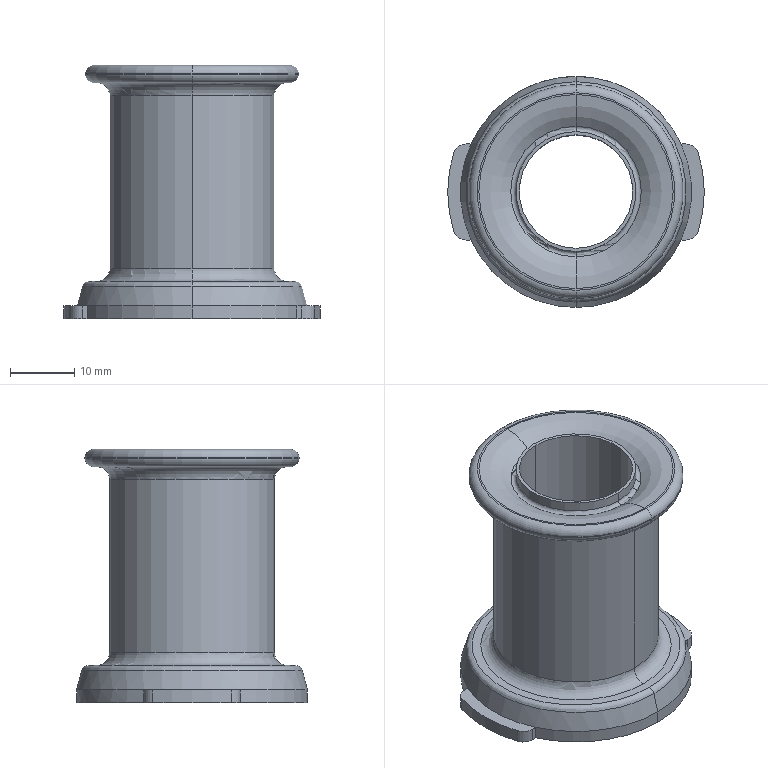Part | SolidWorks | features BaseBody 1 | 1 solid | 51 faces | box 40 x 36 x 39.5 mm | volume 12667 mm3 | cylinder 19 | torus 18 | plane 12 | cone 2 | commonest cylinder face diameters 4 x4 36 x3 17.7 x2 18.7 x2 25.7 x2 33.4 x2
STEP:
#1=CARTESIAN_POINT('',(2003.,227.,823.));
#2=VERTEX_POINT('',#1);
#3=CARTESIAN_POINT('',(2019.363,237.5,823.));
#4=VERTEX_POINT('',#3);
#5=CARTESIAN_POINT('',(2003.,245.,823.));
#6=DIRECTION('',(0.,0.,1.));
#7=DIRECTION('',(0.,-1.,0.));
#8=AXIS2_PLACEMENT_3D('',#5,#6,#7);
#9=CIRCLE('',#8,18.);
#10=EDGE_CURVE('',#2,#4,#9,.T.);
#11=ORIENTED_EDGE('',*,*,#10,.F.);
#12=CARTESIAN_POINT('',(2003.,227.,821.));
#13=VERTEX_POINT('',#12);
#14=CARTESIAN_POINT('',(2003.,227.,862.625));
#15=DIRECTION('',(0.,0.,-1.));
#16=VECTOR('',#15,1000.);
#17=LINE('',#14,#16);
#18=EDGE_CURVE('',#2,#13,#17,.T.);
#19=ORIENTED_EDGE('',*,*,#18,.T.);
#20=CARTESIAN_POINT('',(2019.363,237.5,821.));
#21=VERTEX_POINT('',#20);
#22=CARTESIAN_POINT('',(2003.,245.,821.));
#23=DIRECTION('',(0.,0.,-1.));
#24=DIRECTION('',(0.9091,-0.4167,0.));
#25=AXIS2_PLACEMENT_3D('',#22,#23,#24);
#26=CIRCLE('',#25,18.);
#27=EDGE_CURVE('',#21,#13,#26,.T.);
#28=ORIENTED_EDGE('',*,*,#27,.F.);
#29=CARTESIAN_POINT('',(2019.363,237.5,823.));
#30=DIRECTION('',(0.,0.,-1.));
#31=VECTOR('',#30,1000.);
#32=LINE('',#29,#31);
#33=EDGE_CURVE('',#4,#21,#32,.T.);
#34=ORIENTED_EDGE('',*,*,#33,.F.);
#35=EDGE_LOOP('',(#11,#19,#28,#34));
#36=FACE_OUTER_BOUND('',#35,.T.);
#37=CARTESIAN_POINT('',(2003.,245.,862.625));
#38=DIRECTION('',(0.,0.,-1.));
#39=DIRECTION('',(0.,-1.,0.));
#40=AXIS2_PLACEMENT_3D('',#37,#38,#39);
#41=CYLINDRICAL_SURFACE('',#40,18.);
#42=ADVANCED_FACE('',(#36),#41,.T.);
#43=CARTESIAN_POINT('',(2003.,232.15,823.));
#44=VERTEX_POINT('',#43);
#45=CARTESIAN_POINT('',(2003.,257.85,823.));
#46=VERTEX_POINT('',#45);
#47=CARTESIAN_POINT('',(2003.,245.,823.));
#48=DIRECTION('',(0.,0.,-1.));
#49=DIRECTION('',(0.,-1.,0.));
#50=AXIS2_PLACEMENT_3D('',#47,#48,#49);
#51=CIRCLE('',#50,12.85);
#52=EDGE_CURVE('',#44,#46,#51,.T.);
#53=ORIENTED_EDGE('',*,*,#52,.T.);
#54=CARTESIAN_POINT('',(2003.,253.85,827.));
#55=VERTEX_POINT('',#54);
#56=CARTESIAN_POINT('',(2003.,257.85,827.));
#57=DIRECTION('',(-1.,0.,0.));
#58=DIRECTION('',(0.,-1.,0.));
#59=AXIS2_PLACEMENT_3D('',#56,#57,#58);
#60=CIRCLE('',#59,4.);
#61=EDGE_CURVE('',#46,#55,#60,.T.);
#62=ORIENTED_EDGE('',*,*,#61,.T.);
#63=CARTESIAN_POINT('',(2003.,236.15,827.));
#64=VERTEX_POINT('',#63);
#65=CARTESIAN_POINT('',(2003.,245.,827.));
#66=DIRECTION('',(0.,0.,-1.));
#67=DIRECTION('',(0.,-1.,0.));
#68=AXIS2_PLACEMENT_3D('',#65,#66,#67);
#69=CIRCLE('',#68,8.85);
#70=EDGE_CURVE('',#64,#55,#69,.T.);
#71=ORIENTED_EDGE('',*,*,#70,.F.);
#72=CARTESIAN_POINT('',(2003.,232.15,827.));
#73=DIRECTION('',(-1.,0.,0.));
#74=DIRECTION('',(0.,1.,0.));
#75=AXIS2_PLACEMENT_3D('',#72,#73,#74);
#76=CIRCLE('',#75,4.);
#77=EDGE_CURVE('',#64,#44,#76,.T.);
#78=ORIENTED_EDGE('',*,*,#77,.T.);
#79=EDGE_LOOP('',(#53,#62,#71,#78));
#80=FACE_OUTER_BOUND('',#79,.T.);
#81=CARTESIAN_POINT('',(2003.,245.,827.));
#82=DIRECTION('',(0.,0.,-1.));
#83=DIRECTION('',(0.,-1.,0.));
#84=AXIS2_PLACEMENT_3D('',#81,#82,#83);
#85=TOROIDAL_SURFACE('',#84,12.85,4.);
#86=ADVANCED_FACE('',(#80),#85,.T.);
#87=CARTESIAN_POINT('',(2003.,245.,827.));
#88=DIRECTION('',(0.,0.,1.));
#89=DIRECTION('',(0.,-1.,0.));
#90=AXIS2_PLACEMENT_3D('',#87,#88,#89);
#91=CIRCLE('',#90,8.85);
#92=EDGE_CURVE('',#64,#55,#91,.T.);
#93=ORIENTED_EDGE('',*,*,#92,.T.);
#94=ORIENTED_EDGE('',*,*,#61,.F.);
#95=CARTESIAN_POINT('',(2003.,245.,823.));
#96=DIRECTION('',(0.,0.,1.));
#97=DIRECTION('',(0.,-1.,0.));
#98=AXIS2_PLACEMENT_3D('',#95,#96,#97);
#99=CIRCLE('',#98,12.85);
#100=EDGE_CURVE('',#44,#46,#99,.T.);
#101=ORIENTED_EDGE('',*,*,#100,.F.);
#102=ORIENTED_EDGE('',*,*,#77,.F.);
#103=EDGE_LOOP('',(#93,#94,#101,#102));
#104=FACE_OUTER_BOUND('',#103,.T.);
#105=CARTESIAN_POINT('',(2003.,245.,827.));
#106=DIRECTION('',(0.,0.,-1.));
#107=DIRECTION('',(0.,-1.,0.));
#108=AXIS2_PLACEMENT_3D('',#105,#106,#107);
#109=TOROIDAL_SURFACE('',#108,12.85,4.);
#110=ADVANCED_FACE('',(#104),#109,.T.);
#111=CARTESIAN_POINT('',(2003.,228.5,823.));
#112=VERTEX_POINT('',#111);
#113=CARTESIAN_POINT('',(2003.,261.5,823.));
#114=VERTEX_POINT('',#113);
#115=CARTESIAN_POINT('',(2003.,245.,823.));
#116=DIRECTION('',(0.,0.,1.));
#117=DIRECTION('',(0.,-1.,0.));
#118=AXIS2_PLACEMENT_3D('',#115,#116,#117);
#119=CIRCLE('',#118,16.5);
#120=EDGE_CURVE('',#112,#114,#119,.T.);
#121=ORIENTED_EDGE('',*,*,#120,.F.);
#122=CARTESIAN_POINT('',(2003.,245.,823.));
#123=DIRECTION('',(0.,0.,-1.));
#124=DIRECTION('',(0.,-1.,0.));
#125=AXIS2_PLACEMENT_3D('',#122,#123,#124);
#126=CIRCLE('',#125,16.5);
#127=EDGE_CURVE('',#112,#114,#126,.T.);
#128=ORIENTED_EDGE('',*,*,#127,.T.);
#129=EDGE_LOOP('',(#121,#128));
#130=FACE_OUTER_BOUND('',#129,.T.);
#131=ORIENTED_EDGE('',*,*,#52,.F.);
#132=ORIENTED_EDGE('',*,*,#100,.T.);
#133=EDGE_LOOP('',(#131,#132));
#134=FACE_BOUND('',#133,.T.);
#135=CARTESIAN_POINT('',(2003.,245.,823.));
#136=DIRECTION('',(0.,0.,-1.));
#137=DIRECTION('',(0.,-1.,0.));
#138=AXIS2_PLACEMENT_3D('',#135,#136,#137);
#139=PLANE('',#138);
#140=ADVANCED_FACE('',(#130,#134),#139,.T.);
#141=CARTESIAN_POINT('',(2003.,227.5,822.));
#142=VERTEX_POINT('',#141);
#143=CARTESIAN_POINT('',(2003.,262.5,822.));
#144=VERTEX_POINT('',#143);
#145=CARTESIAN_POINT('',(2003.,245.,822.));
#146=DIRECTION('',(0.,0.,-1.));
#147=DIRECTION('',(0.,-1.,0.));
#148=AXIS2_PLACEMENT_3D('',#145,#146,#147);
#149=CIRCLE('',#148,17.5);
#150=EDGE_CURVE('',#142,#144,#149,.T.);
#151=ORIENTED_EDGE('',*,*,#150,.T.);
#152=CARTESIAN_POINT('',(2003.,261.5,822.));
#153=DIRECTION('',(1.,0.,0.));
#154=DIRECTION('',(0.,0.,1.));
#155=AXIS2_PLACEMENT_3D('',#152,#153,#154);
#156=CIRCLE('',#155,1.);
#157=EDGE_CURVE('',#144,#114,#156,.T.);
#158=ORIENTED_EDGE('',*,*,#157,.T.);
#159=ORIENTED_EDGE('',*,*,#127,.F.);
#160=CARTESIAN_POINT('',(2003.,228.5,822.));
#161=DIRECTION('',(1.,0.,0.));
#162=DIRECTION('',(0.,0.,1.));
#163=AXIS2_PLACEMENT_3D('',#160,#161,#162);
#164=CIRCLE('',#163,1.);
#165=EDGE_CURVE('',#112,#142,#164,.T.);
#166=ORIENTED_EDGE('',*,*,#165,.T.);
#167=EDGE_LOOP('',(#151,#158,#159,#166));
#168=FACE_OUTER_BOUND('',#167,.T.);
#169=CARTESIAN_POINT('',(2003.,245.,822.));
#170=DIRECTION('',(0.,0.,-1.));
#171=DIRECTION('',(0.,-1.,0.));
#172=AXIS2_PLACEMENT_3D('',#169,#170,#171);
#173=TOROIDAL_SURFACE('',#172,16.5,1.);
#174=ADVANCED_FACE('',(#168),#173,.F.);
#175=ORIENTED_EDGE('',*,*,#120,.T.);
#176=ORIENTED_EDGE('',*,*,#157,.F.);
#177=CARTESIAN_POINT('',(2003.,245.,822.));
#178=DIRECTION('',(0.,0.,1.));
#179=DIRECTION('',(0.,-1.,0.));
#180=AXIS2_PLACEMENT_3D('',#177,#178,#179);
#181=CIRCLE('',#180,17.5);
#182=EDGE_CURVE('',#142,#144,#181,.T.);
#183=ORIENTED_EDGE('',*,*,#182,.F.);
#184=ORIENTED_EDGE('',*,*,#165,.F.);
#185=EDGE_LOOP('',(#175,#176,#183,#184));
#186=FACE_OUTER_BOUND('',#185,.T.);
#187=CARTESIAN_POINT('',(2003.,245.,822.));
#188=DIRECTION('',(0.,0.,-1.));
#189=DIRECTION('',(0.,-1.,0.));
#190=AXIS2_PLACEMENT_3D('',#187,#188,#189);
#191=TOROIDAL_SURFACE('',#190,16.5,1.);
#192=ADVANCED_FACE('',(#186),#191,.F.);
#193=CARTESIAN_POINT('',(2003.,227.5,821.));
#194=VERTEX_POINT('',#193);
#195=CARTESIAN_POINT('',(2003.,227.5,822.));
#196=DIRECTION('',(0.,0.,1.));
#197=VECTOR('',#196,1000.);
#198=LINE('',#195,#197);
#199=EDGE_CURVE('',#194,#142,#198,.T.);
#200=ORIENTED_EDGE('',*,*,#199,.T.);
#201=ORIENTED_EDGE('',*,*,#182,.T.);
#202=CARTESIAN_POINT('',(2003.,262.5,821.));
#203=VERTEX_POINT('',#202);
#204=CARTESIAN_POINT('',(2003.,262.5,822.));
#205=DIRECTION('',(0.,0.,-1.));
#206=VECTOR('',#205,1000.);
#207=LINE('',#204,#206);
#208=EDGE_CURVE('',#144,#203,#207,.T.);
#209=ORIENTED_EDGE('',*,*,#208,.T.);
#210=CARTESIAN_POINT('',(2003.,245.,821.));
#211=DIRECTION('',(0.,0.,-1.));
#212=DIRECTION('',(0.,1.,0.));
#213=AXIS2_PLACEMENT_3D('',#210,#211,#212);
#214=CIRCLE('',#213,17.5);
#215=EDGE_CURVE('',#203,#194,#214,.T.);
#216=ORIENTED_EDGE('',*,*,#215,.T.);
#217=EDGE_LOOP('',(#200,#201,#209,#216));
#218=FACE_OUTER_BOUND('',#217,.T.);
#219=CARTESIAN_POINT('',(2003.,245.,862.625));
#220=DIRECTION('',(0.,0.,-1.));
#221=DIRECTION('',(0.,-1.,0.));
#222=AXIS2_PLACEMENT_3D('',#219,#220,#221);
#223=CYLINDRICAL_SURFACE('',#222,17.5);
#224=ADVANCED_FACE('',(#218),#223,.F.);
#225=CARTESIAN_POINT('',(1985.861,237.5,821.));
#226=VERTEX_POINT('',#225);
#227=CARTESIAN_POINT('',(1986.637,237.5,821.));
#228=VERTEX_POINT('',#227);
#229=CARTESIAN_POINT('',(1985.861,237.5,821.));
#230=DIRECTION('',(1.,0.,0.));
#231=VECTOR('',#230,1000.);
#232=LINE('',#229,#231);
#233=EDGE_CURVE('',#226,#228,#232,.T.);
#234=ORIENTED_EDGE('',*,*,#233,.F.);
#235=CARTESIAN_POINT('',(1983.957,238.889,821.));
#236=VERTEX_POINT('',#235);
#237=CARTESIAN_POINT('',(1985.861,239.5,821.));
#238=DIRECTION('',(0.,0.,1.));
#239=DIRECTION('',(-0.9522,-0.3056,0.));
#240=AXIS2_PLACEMENT_3D('',#237,#238,#239);
#241=CIRCLE('',#240,2.);
#242=EDGE_CURVE('',#236,#226,#241,.T.);
#243=ORIENTED_EDGE('',*,*,#242,.F.);
#244=CARTESIAN_POINT('',(1983.957,251.111,821.));
#245=VERTEX_POINT('',#244);
#246=CARTESIAN_POINT('',(2003.,245.,821.));
#247=DIRECTION('',(0.,0.,1.));
#248=DIRECTION('',(-0.9522,0.3056,0.));
#249=AXIS2_PLACEMENT_3D('',#246,#247,#248);
#250=CIRCLE('',#249,20.);
#251=EDGE_CURVE('',#245,#236,#250,.T.);
#252=ORIENTED_EDGE('',*,*,#251,.F.);
#253=CARTESIAN_POINT('',(1985.861,252.5,821.));
#254=VERTEX_POINT('',#253);
#255=CARTESIAN_POINT('',(1985.861,250.5,821.));
#256=DIRECTION('',(0.,0.,1.));
#257=DIRECTION('',(0.,1.,0.));
#258=AXIS2_PLACEMENT_3D('',#255,#256,#257);
#259=CIRCLE('',#258,2.);
#260=EDGE_CURVE('',#254,#245,#259,.T.);
#261=ORIENTED_EDGE('',*,*,#260,.F.);
#262=CARTESIAN_POINT('',(1986.637,252.5,821.));
#263=VERTEX_POINT('',#262);
#264=CARTESIAN_POINT('',(1986.637,252.5,821.));
#265=DIRECTION('',(-1.,0.,0.));
#266=VECTOR('',#265,1000.);
#267=LINE('',#264,#266);
#268=EDGE_CURVE('',#263,#254,#267,.T.);
#269=ORIENTED_EDGE('',*,*,#268,.F.);
#270=CARTESIAN_POINT('',(2019.363,252.5,821.));
#271=VERTEX_POINT('',#270);
#272=CARTESIAN_POINT('',(2003.,245.,821.));
#273=DIRECTION('',(0.,0.,-1.));
#274=DIRECTION('',(-0.9091,0.4167,0.));
#275=AXIS2_PLACEMENT_3D('',#272,#273,#274);
#276=CIRCLE('',#275,18.);
#277=EDGE_CURVE('',#263,#271,#276,.T.);
#278=ORIENTED_EDGE('',*,*,#277,.T.);
#279=CARTESIAN_POINT('',(2020.139,252.5,821.));
#280=VERTEX_POINT('',#279);
#281=CARTESIAN_POINT('',(2020.139,252.5,821.));
#282=DIRECTION('',(-1.,0.,0.));
#283=VECTOR('',#282,1000.);
#284=LINE('',#281,#283);
#285=EDGE_CURVE('',#280,#271,#284,.T.);
#286=ORIENTED_EDGE('',*,*,#285,.F.);
#287=CARTESIAN_POINT('',(2022.043,251.111,821.));
#288=VERTEX_POINT('',#287);
#289=CARTESIAN_POINT('',(2020.139,250.5,821.));
#290=DIRECTION('',(0.,0.,1.));
#291=DIRECTION('',(0.9522,0.3056,0.));
#292=AXIS2_PLACEMENT_3D('',#289,#290,#291);
#293=CIRCLE('',#292,2.);
#294=EDGE_CURVE('',#288,#280,#293,.T.);
#295=ORIENTED_EDGE('',*,*,#294,.F.);
#296=CARTESIAN_POINT('',(2022.043,238.889,821.));
#297=VERTEX_POINT('',#296);
#298=CARTESIAN_POINT('',(2003.,245.,821.));
#299=DIRECTION('',(0.,0.,1.));
#300=DIRECTION('',(0.9522,-0.3056,0.));
#301=AXIS2_PLACEMENT_3D('',#298,#299,#300);
#302=CIRCLE('',#301,20.);
#303=EDGE_CURVE('',#297,#288,#302,.T.);
#304=ORIENTED_EDGE('',*,*,#303,.F.);
#305=CARTESIAN_POINT('',(2020.139,237.5,821.));
#306=VERTEX_POINT('',#305);
#307=CARTESIAN_POINT('',(2020.139,239.5,821.));
#308=DIRECTION('',(0.,0.,1.));
#309=DIRECTION('',(0.,-1.,0.));
#310=AXIS2_PLACEMENT_3D('',#307,#308,#309);
#311=CIRCLE('',#310,2.);
#312=EDGE_CURVE('',#306,#297,#311,.T.);
#313=ORIENTED_EDGE('',*,*,#312,.F.);
#314=CARTESIAN_POINT('',(2019.363,237.5,821.));
#315=DIRECTION('',(1.,0.,0.));
#316=VECTOR('',#315,1000.);
#317=LINE('',#314,#316);
#318=EDGE_CURVE('',#21,#306,#317,.T.);
#319=ORIENTED_EDGE('',*,*,#318,.F.);
#320=ORIENTED_EDGE('',*,*,#27,.T.);
#321=CARTESIAN_POINT('',(2003.,245.,821.));
#322=DIRECTION('',(0.,0.,-1.));
#323=DIRECTION('',(0.9091,-0.4167,0.));
#324=AXIS2_PLACEMENT_3D('',#321,#322,#323);
#325=CIRCLE('',#324,18.);
#326=EDGE_CURVE('',#13,#228,#325,.T.);
#327=ORIENTED_EDGE('',*,*,#326,.T.);
#328=EDGE_LOOP('',(#234,#243,#252,#261,#269,#278,#286,#295,#304,#313,#319,#320,#327));
#329=FACE_OUTER_BOUND('',#328,.T.);
#330=ORIENTED_EDGE('',*,*,#215,.F.);
#331=CARTESIAN_POINT('',(2003.,245.,821.));
#332=DIRECTION('',(0.,0.,-1.));
#333=DIRECTION('',(0.,-1.,0.));
#334=AXIS2_PLACEMENT_3D('',#331,#332,#333);
#335=CIRCLE('',#334,17.5);
#336=EDGE_CURVE('',#194,#203,#335,.T.);
#337=ORIENTED_EDGE('',*,*,#336,.F.);
#338=EDGE_LOOP('',(#330,#337));
#339=FACE_BOUND('',#338,.T.);
#340=CARTESIAN_POINT('',(1979.27,266.6,821.));
#341=DIRECTION('',(0.,0.,1.));
#342=DIRECTION('',(-1.,0.,0.));
#343=AXIS2_PLACEMENT_3D('',#340,#341,#342);
#344=PLANE('',#343);
#345=ADVANCED_FACE('',(#329,#339),#344,.F.);
#346=ORIENTED_EDGE('',*,*,#208,.F.);
#347=ORIENTED_EDGE('',*,*,#150,.F.);
#348=ORIENTED_EDGE('',*,*,#199,.F.);
#349=ORIENTED_EDGE('',*,*,#336,.T.);
#350=EDGE_LOOP('',(#346,#347,#348,#349));
#351=FACE_OUTER_BOUND('',#350,.T.);
#352=CARTESIAN_POINT('',(2003.,245.,862.625));
#353=DIRECTION('',(0.,0.,-1.));
#354=DIRECTION('',(0.,-1.,0.));
#355=AXIS2_PLACEMENT_3D('',#352,#353,#354);
#356=CYLINDRICAL_SURFACE('',#355,17.5);
#357=ADVANCED_FACE('',(#351),#356,.F.);
#358=ORIENTED_EDGE('',*,*,#18,.F.);
#359=CARTESIAN_POINT('',(1986.637,237.5,823.));
#360=VERTEX_POINT('',#359);
#361=CARTESIAN_POINT('',(2003.,245.,823.));
#362=DIRECTION('',(0.,0.,-1.));
#363=DIRECTION('',(0.,-1.,0.));
#364=AXIS2_PLACEMENT_3D('',#361,#362,#363);
#365=CIRCLE('',#364,18.);
#366=EDGE_CURVE('',#2,#360,#365,.T.);
#367=ORIENTED_EDGE('',*,*,#366,.T.);
#368=CARTESIAN_POINT('',(1986.637,237.5,823.));
#369=DIRECTION('',(0.,0.,-1.));
#370=VECTOR('',#369,1000.);
#371=LINE('',#368,#370);
#372=EDGE_CURVE('',#360,#228,#371,.T.);
#373=ORIENTED_EDGE('',*,*,#372,.T.);
#374=ORIENTED_EDGE('',*,*,#326,.F.);
#375=EDGE_LOOP('',(#358,#367,#373,#374));
#376=FACE_OUTER_BOUND('',#375,.T.);
#377=CARTESIAN_POINT('',(2003.,245.,862.625));
#378=DIRECTION('',(0.,0.,-1.));
#379=DIRECTION('',(0.,-1.,0.));
#380=AXIS2_PLACEMENT_3D('',#377,#378,#379);
#381=CYLINDRICAL_SURFACE('',#380,18.);
#382=ADVANCED_FACE('',(#376),#381,.T.);
#383=CARTESIAN_POINT('',(1986.637,252.5,823.));
#384=VERTEX_POINT('',#383);
#385=CARTESIAN_POINT('',(1986.637,252.5,823.));
#386=DIRECTION('',(0.,0.,-1.));
#387=VECTOR('',#386,1000.);
#388=LINE('',#385,#387);
#389=EDGE_CURVE('',#384,#263,#388,.T.);
#390=ORIENTED_EDGE('',*,*,#389,.F.);
#391=CARTESIAN_POINT('',(2003.,263.,823.));
#392=VERTEX_POINT('',#391);
#393=CARTESIAN_POINT('',(2003.,245.,823.));
#394=DIRECTION('',(0.,0.,-1.));
#395=DIRECTION('',(-0.9091,0.4167,0.));
#396=AXIS2_PLACEMENT_3D('',#393,#394,#395);
#397=CIRCLE('',#396,18.);
#398=EDGE_CURVE('',#384,#392,#397,.T.);
#399=ORIENTED_EDGE('',*,*,#398,.T.);
#400=CARTESIAN_POINT('',(2019.363,252.5,823.));
#401=VERTEX_POINT('',#400);
#402=CARTESIAN_POINT('',(2003.,245.,823.));
#403=DIRECTION('',(0.,0.,1.));
#404=DIRECTION('',(0.9091,0.4167,0.));
#405=AXIS2_PLACEMENT_3D('',#402,#403,#404);
#406=CIRCLE('',#405,18.);
#407=EDGE_CURVE('',#401,#392,#406,.T.);
#408=ORIENTED_EDGE('',*,*,#407,.F.);
#409=CARTESIAN_POINT('',(2019.363,252.5,823.));
#410=DIRECTION('',(0.,0.,-1.));
#411=VECTOR('',#410,1000.);
#412=LINE('',#409,#411);
#413=EDGE_CURVE('',#401,#271,#412,.T.);
#414=ORIENTED_EDGE('',*,*,#413,.T.);
#415=ORIENTED_EDGE('',*,*,#277,.F.);
#416=EDGE_LOOP('',(#390,#399,#408,#414,#415));
#417=FACE_OUTER_BOUND('',#416,.T.);
#418=CARTESIAN_POINT('',(2003.,245.,862.625));
#419=DIRECTION('',(0.,0.,-1.));
#420=DIRECTION('',(0.,-1.,0.));
#421=AXIS2_PLACEMENT_3D('',#418,#419,#420);
#422=CYLINDRICAL_SURFACE('',#421,18.);
#423=ADVANCED_FACE('',(#417),#422,.T.);
#424=ORIENTED_EDGE('',*,*,#366,.F.);
#425=CARTESIAN_POINT('',(2003.,227.82,826.059));
#426=VERTEX_POINT('',#425);
#427=CARTESIAN_POINT('',(2003.,227.,823.));
#428=DIRECTION('',(0.,0.2588,0.9659));
#429=VECTOR('',#428,1000.);
#430=LINE('',#427,#429);
#431=EDGE_CURVE('',#2,#426,#430,.T.);
#432=ORIENTED_EDGE('',*,*,#431,.T.);
#433=CARTESIAN_POINT('',(2003.,262.18,826.059));
#434=VERTEX_POINT('',#433);
#435=CARTESIAN_POINT('',(2003.,245.,826.059));
#436=DIRECTION('',(0.,0.,-1.));
#437=DIRECTION('',(0.,-1.,0.));
#438=AXIS2_PLACEMENT_3D('',#435,#436,#437);
#439=CIRCLE('',#438,17.18);
#440=EDGE_CURVE('',#426,#434,#439,.T.);
#441=ORIENTED_EDGE('',*,*,#440,.T.);
#442=CARTESIAN_POINT('',(2003.,263.,823.));
#443=DIRECTION('',(0.,0.2588,-0.9659));
#444=VECTOR('',#443,1000.);
#445=LINE('',#442,#444);
#446=EDGE_CURVE('',#434,#392,#445,.T.);
#447=ORIENTED_EDGE('',*,*,#446,.T.);
#448=ORIENTED_EDGE('',*,*,#398,.F.);
#449=CARTESIAN_POINT('',(2003.,245.,823.));
#450=DIRECTION('',(0.,0.,-1.));
#451=DIRECTION('',(-0.9091,-0.4167,0.));
#452=AXIS2_PLACEMENT_3D('',#449,#450,#451);
#453=CIRCLE('',#452,18.);
#454=EDGE_CURVE('',#360,#384,#453,.T.);
#455=ORIENTED_EDGE('',*,*,#454,.F.);
#456=EDGE_LOOP('',(#424,#432,#441,#447,#448,#455));
#457=FACE_OUTER_BOUND('',#456,.T.);
#458=CARTESIAN_POINT('',(2003.,245.,824.529));
#459=DIRECTION('',(0.,0.,-1.));
#460=DIRECTION('',(0.,-1.,0.));
#461=AXIS2_PLACEMENT_3D('',#458,#459,#460);
#462=CONICAL_SURFACE('',#461,17.59,0.2618);
#463=ADVANCED_FACE('',(#457),#462,.T.);
#464=CARTESIAN_POINT('',(1985.861,252.5,823.));
#465=VERTEX_POINT('',#464);
#466=CARTESIAN_POINT('',(1986.637,252.5,823.));
#467=DIRECTION('',(-1.,0.,0.));
#468=VECTOR('',#467,1000.);
#469=LINE('',#466,#468);
#470=EDGE_CURVE('',#384,#465,#469,.T.);
#471=ORIENTED_EDGE('',*,*,#470,.T.);
#472=CARTESIAN_POINT('',(1983.957,251.111,823.));
#473=VERTEX_POINT('',#472);
#474=CARTESIAN_POINT('',(1985.861,250.5,823.));
#475=DIRECTION('',(0.,0.,1.));
#476=DIRECTION('',(0.,1.,0.));
#477=AXIS2_PLACEMENT_3D('',#474,#475,#476);
#478=CIRCLE('',#477,2.);
#479=EDGE_CURVE('',#465,#473,#478,.T.);
#480=ORIENTED_EDGE('',*,*,#479,.T.);
#481=CARTESIAN_POINT('',(1983.957,238.889,823.));
#482=VERTEX_POINT('',#481);
#483=CARTESIAN_POINT('',(2003.,245.,823.));
#484=DIRECTION('',(0.,0.,1.));
#485=DIRECTION('',(-0.9522,0.3056,0.));
#486=AXIS2_PLACEMENT_3D('',#483,#484,#485);
#487=CIRCLE('',#486,20.);
#488=EDGE_CURVE('',#473,#482,#487,.T.);
#489=ORIENTED_EDGE('',*,*,#488,.T.);
#490=CARTESIAN_POINT('',(1985.861,237.5,823.));
#491=VERTEX_POINT('',#490);
#492=CARTESIAN_POINT('',(1985.861,239.5,823.));
#493=DIRECTION('',(0.,0.,1.));
#494=DIRECTION('',(-0.9522,-0.3056,0.));
#495=AXIS2_PLACEMENT_3D('',#492,#493,#494);
#496=CIRCLE('',#495,2.);
#497=EDGE_CURVE('',#482,#491,#496,.T.);
#498=ORIENTED_EDGE('',*,*,#497,.T.);
#499=CARTESIAN_POINT('',(1985.861,237.5,823.));
#500=DIRECTION('',(1.,0.,0.));
#501=VECTOR('',#500,1000.);
#502=LINE('',#499,#501);
#503=EDGE_CURVE('',#491,#360,#502,.T.);
#504=ORIENTED_EDGE('',*,*,#503,.T.);
#505=ORIENTED_EDGE('',*,*,#454,.T.);
#506=EDGE_LOOP('',(#471,#480,#489,#498,#504,#505));
#507=FACE_OUTER_BOUND('',#506,.T.);
#508=CARTESIAN_POINT('',(2003.,245.,823.));
#509=DIRECTION('',(0.,0.,1.));
#510=DIRECTION('',(0.,-1.,0.));
#511=AXIS2_PLACEMENT_3D('',#508,#509,#510);
#512=PLANE('',#511);
#513=ADVANCED_FACE('',(#507),#512,.T.);
#514=CARTESIAN_POINT('',(2020.139,237.5,823.));
#515=VERTEX_POINT('',#514);
#516=CARTESIAN_POINT('',(2019.363,237.5,823.));
#517=DIRECTION('',(1.,0.,0.));
#518=VECTOR('',#517,1000.);
#519=LINE('',#516,#518);
#520=EDGE_CURVE('',#4,#515,#519,.T.);
#521=ORIENTED_EDGE('',*,*,#520,.T.);
#522=CARTESIAN_POINT('',(2022.043,238.889,823.));
#523=VERTEX_POINT('',#522);
#524=CARTESIAN_POINT('',(2020.139,239.5,823.));
#525=DIRECTION('',(0.,0.,1.));
#526=DIRECTION('',(0.,-1.,0.));
#527=AXIS2_PLACEMENT_3D('',#524,#525,#526);
#528=CIRCLE('',#527,2.);
#529=EDGE_CURVE('',#515,#523,#528,.T.);
#530=ORIENTED_EDGE('',*,*,#529,.T.);
#531=CARTESIAN_POINT('',(2022.043,251.111,823.));
#532=VERTEX_POINT('',#531);
#533=CARTESIAN_POINT('',(2003.,245.,823.));
#534=DIRECTION('',(0.,0.,1.));
#535=DIRECTION('',(0.9522,-0.3056,0.));
#536=AXIS2_PLACEMENT_3D('',#533,#534,#535);
#537=CIRCLE('',#536,20.);
#538=EDGE_CURVE('',#523,#532,#537,.T.);
#539=ORIENTED_EDGE('',*,*,#538,.T.);
#540=CARTESIAN_POINT('',(2020.139,252.5,823.));
#541=VERTEX_POINT('',#540);
#542=CARTESIAN_POINT('',(2020.139,250.5,823.));
#543=DIRECTION('',(0.,0.,1.));
#544=DIRECTION('',(0.9522,0.3056,0.));
#545=AXIS2_PLACEMENT_3D('',#542,#543,#544);
#546=CIRCLE('',#545,2.);
#547=EDGE_CURVE('',#532,#541,#546,.T.);
#548=ORIENTED_EDGE('',*,*,#547,.T.);
#549=CARTESIAN_POINT('',(2020.139,252.5,823.));
#550=DIRECTION('',(-1.,0.,0.));
#551=VECTOR('',#550,1000.);
#552=LINE('',#549,#551);
#553=EDGE_CURVE('',#541,#401,#552,.T.);
#554=ORIENTED_EDGE('',*,*,#553,.T.);
#555=CARTESIAN_POINT('',(2003.,245.,823.));
#556=DIRECTION('',(0.,0.,-1.));
#557=DIRECTION('',(0.9091,0.4167,0.));
#558=AXIS2_PLACEMENT_3D('',#555,#556,#557);
#559=CIRCLE('',#558,18.);
#560=EDGE_CURVE('',#401,#4,#559,.T.);
#561=ORIENTED_EDGE('',*,*,#560,.T.);
#562=EDGE_LOOP('',(#521,#530,#539,#548,#554,#561));
#563=FACE_OUTER_BOUND('',#562,.T.);
#564=CARTESIAN_POINT('',(2003.,245.,823.));
#565=DIRECTION('',(0.,0.,1.));
#566=DIRECTION('',(0.,-1.,0.));
#567=AXIS2_PLACEMENT_3D('',#564,#565,#566);
#568=PLANE('',#567);
#569=ADVANCED_FACE('',(#563),#568,.T.);
#570=ORIENTED_EDGE('',*,*,#372,.F.);
#571=ORIENTED_EDGE('',*,*,#503,.F.);
#572=CARTESIAN_POINT('',(1985.861,237.5,821.));
#573=DIRECTION('',(0.,0.,1.));
#574=VECTOR('',#573,1000.);
#575=LINE('',#572,#574);
#576=EDGE_CURVE('',#226,#491,#575,.T.);
#577=ORIENTED_EDGE('',*,*,#576,.F.);
#578=ORIENTED_EDGE('',*,*,#233,.T.);
#579=EDGE_LOOP('',(#570,#571,#577,#578));
#580=FACE_OUTER_BOUND('',#579,.T.);
#581=CARTESIAN_POINT('',(1985.861,237.5,819.));
#582=DIRECTION('',(0.,-1.,0.));
#583=DIRECTION('',(-1.,0.,0.));
#584=AXIS2_PLACEMENT_3D('',#581,#582,#583);
#585=PLANE('',#584);
#586=ADVANCED_FACE('',(#580),#585,.T.);
#587=ORIENTED_EDGE('',*,*,#576,.T.);
#588=ORIENTED_EDGE('',*,*,#497,.F.);
#589=CARTESIAN_POINT('',(1983.957,238.889,821.));
#590=DIRECTION('',(0.,0.,1.));
#591=VECTOR('',#590,1000.);
#592=LINE('',#589,#591);
#593=EDGE_CURVE('',#236,#482,#592,.T.);
#594=ORIENTED_EDGE('',*,*,#593,.F.);
#595=ORIENTED_EDGE('',*,*,#242,.T.);
#596=EDGE_LOOP('',(#587,#588,#594,#595));
#597=FACE_OUTER_BOUND('',#596,.T.);
#598=CARTESIAN_POINT('',(1985.861,239.5,819.));
#599=DIRECTION('',(0.,0.,1.));
#600=DIRECTION('',(0.,-1.,0.));
#601=AXIS2_PLACEMENT_3D('',#598,#599,#600);
#602=CYLINDRICAL_SURFACE('',#601,2.);
#603=ADVANCED_FACE('',(#597),#602,.T.);
#604=ORIENTED_EDGE('',*,*,#593,.T.);
#605=ORIENTED_EDGE('',*,*,#488,.F.);
#606=CARTESIAN_POINT('',(1983.957,251.111,821.));
#607=DIRECTION('',(0.,0.,1.));
#608=VECTOR('',#607,1000.);
#609=LINE('',#606,#608);
#610=EDGE_CURVE('',#245,#473,#609,.T.);
#611=ORIENTED_EDGE('',*,*,#610,.F.);
#612=ORIENTED_EDGE('',*,*,#251,.T.);
#613=EDGE_LOOP('',(#604,#605,#611,#612));
#614=FACE_OUTER_BOUND('',#613,.T.);
#615=CARTESIAN_POINT('',(2003.,245.,819.));
#616=DIRECTION('',(0.,0.,1.));
#617=DIRECTION('',(0.,-1.,0.));
#618=AXIS2_PLACEMENT_3D('',#615,#616,#617);
#619=CYLINDRICAL_SURFACE('',#618,20.);
#620=ADVANCED_FACE('',(#614),#619,.T.);
#621=ORIENTED_EDGE('',*,*,#610,.T.);
#622=ORIENTED_EDGE('',*,*,#479,.F.);
#623=CARTESIAN_POINT('',(1985.861,252.5,821.));
#624=DIRECTION('',(0.,0.,1.));
#625=VECTOR('',#624,1000.);
#626=LINE('',#623,#625);
#627=EDGE_CURVE('',#254,#465,#626,.T.);
#628=ORIENTED_EDGE('',*,*,#627,.F.);
#629=ORIENTED_EDGE('',*,*,#260,.T.);
#630=EDGE_LOOP('',(#621,#622,#628,#629));
#631=FACE_OUTER_BOUND('',#630,.T.);
#632=CARTESIAN_POINT('',(1985.861,250.5,819.));
#633=DIRECTION('',(0.,0.,1.));
#634=DIRECTION('',(0.,-1.,0.));
#635=AXIS2_PLACEMENT_3D('',#632,#633,#634);
#636=CYLINDRICAL_SURFACE('',#635,2.);
#637=ADVANCED_FACE('',(#631),#636,.T.);
#638=ORIENTED_EDGE('',*,*,#627,.T.);
#639=ORIENTED_EDGE('',*,*,#470,.F.);
#640=ORIENTED_EDGE('',*,*,#389,.T.);
#641=ORIENTED_EDGE('',*,*,#268,.T.);
#642=EDGE_LOOP('',(#638,#639,#640,#641));
#643=FACE_OUTER_BOUND('',#642,.T.);
#644=CARTESIAN_POINT('',(1986.637,252.5,819.));
#645=DIRECTION('',(0.,1.,0.));
#646=DIRECTION('',(1.,0.,0.));
#647=AXIS2_PLACEMENT_3D('',#644,#645,#646);
#648=PLANE('',#647);
#649=ADVANCED_FACE('',(#643),#648,.T.);
#650=ORIENTED_EDGE('',*,*,#407,.T.);
#651=ORIENTED_EDGE('',*,*,#446,.F.);
#652=CARTESIAN_POINT('',(2003.,245.,826.059));
#653=DIRECTION('',(0.,0.,1.));
#654=DIRECTION('',(0.,-1.,0.));
#655=AXIS2_PLACEMENT_3D('',#652,#653,#654);
#656=CIRCLE('',#655,17.18);
#657=EDGE_CURVE('',#426,#434,#656,.T.);
#658=ORIENTED_EDGE('',*,*,#657,.F.);
#659=ORIENTED_EDGE('',*,*,#431,.F.);
#660=ORIENTED_EDGE('',*,*,#10,.T.);
#661=ORIENTED_EDGE('',*,*,#560,.F.);
#662=EDGE_LOOP('',(#650,#651,#658,#659,#660,#661));
#663=FACE_OUTER_BOUND('',#662,.T.);
#664=CARTESIAN_POINT('',(2003.,245.,824.529));
#665=DIRECTION('',(0.,0.,-1.));
#666=DIRECTION('',(0.,-1.,0.));
#667=AXIS2_PLACEMENT_3D('',#664,#665,#666);
#668=CONICAL_SURFACE('',#667,17.59,0.2618);
#669=ADVANCED_FACE('',(#663),#668,.T.);
#670=ORIENTED_EDGE('',*,*,#657,.T.);
#671=CARTESIAN_POINT('',(2003.,261.214,826.8));
#672=VERTEX_POINT('',#671);
#673=CARTESIAN_POINT('',(2003.,261.214,825.8));
#674=DIRECTION('',(1.,0.,0.));
#675=DIRECTION('',(0.,0.9659,0.2588));
#676=AXIS2_PLACEMENT_3D('',#673,#674,#675);
#677=CIRCLE('',#676,1.);
#678=EDGE_CURVE('',#434,#672,#677,.T.);
#679=ORIENTED_EDGE('',*,*,#678,.T.);
#680=CARTESIAN_POINT('',(2003.,228.786,826.8));
#681=VERTEX_POINT('',#680);
#682=CARTESIAN_POINT('',(2003.,245.,826.8));
#683=DIRECTION('',(0.,0.,1.));
#684=DIRECTION('',(0.,-1.,0.));
#685=AXIS2_PLACEMENT_3D('',#682,#683,#684);
#686=CIRCLE('',#685,16.214);
#687=EDGE_CURVE('',#681,#672,#686,.T.);
#688=ORIENTED_EDGE('',*,*,#687,.F.);
#689=CARTESIAN_POINT('',(2003.,228.786,825.8));
#690=DIRECTION('',(1.,0.,0.));
#691=DIRECTION('',(0.,-0.9659,0.2588));
#692=AXIS2_PLACEMENT_3D('',#689,#690,#691);
#693=CIRCLE('',#692,1.);
#694=EDGE_CURVE('',#681,#426,#693,.T.);
#695=ORIENTED_EDGE('',*,*,#694,.T.);
#696=EDGE_LOOP('',(#670,#679,#688,#695));
#697=FACE_OUTER_BOUND('',#696,.T.);
#698=CARTESIAN_POINT('',(2003.,245.,825.8));
#699=DIRECTION('',(0.,0.,-1.));
#700=DIRECTION('',(0.,-1.,0.));
#701=AXIS2_PLACEMENT_3D('',#698,#699,#700);
#702=TOROIDAL_SURFACE('',#701,16.214,1.);
#703=ADVANCED_FACE('',(#697),#702,.T.);
#704=CARTESIAN_POINT('',(2003.,245.,826.8));
#705=DIRECTION('',(0.,0.,-1.));
#706=DIRECTION('',(0.,-1.,0.));
#707=AXIS2_PLACEMENT_3D('',#704,#705,#706);
#708=CIRCLE('',#707,16.214);
#709=EDGE_CURVE('',#681,#672,#708,.T.);
#710=ORIENTED_EDGE('',*,*,#709,.T.);
#711=ORIENTED_EDGE('',*,*,#678,.F.);
#712=ORIENTED_EDGE('',*,*,#440,.F.);
#713=ORIENTED_EDGE('',*,*,#694,.F.);
#714=EDGE_LOOP('',(#710,#711,#712,#713));
#715=FACE_OUTER_BOUND('',#714,.T.);
#716=CARTESIAN_POINT('',(2003.,245.,825.8));
#717=DIRECTION('',(0.,0.,-1.));
#718=DIRECTION('',(0.,-1.,0.));
#719=AXIS2_PLACEMENT_3D('',#716,#717,#718);
#720=TOROIDAL_SURFACE('',#719,16.214,1.);
#721=ADVANCED_FACE('',(#715),#720,.T.);
#722=ORIENTED_EDGE('',*,*,#709,.F.);
#723=ORIENTED_EDGE('',*,*,#687,.T.);
#724=EDGE_LOOP('',(#722,#723));
#725=FACE_OUTER_BOUND('',#724,.T.);
#726=CARTESIAN_POINT('',(2003.,230.15,826.8));
#727=VERTEX_POINT('',#726);
#728=CARTESIAN_POINT('',(2003.,259.85,826.8));
#729=VERTEX_POINT('',#728);
#730=CARTESIAN_POINT('',(2003.,245.,826.8));
#731=DIRECTION('',(0.,0.,1.));
#732=DIRECTION('',(0.,-1.,0.));
#733=AXIS2_PLACEMENT_3D('',#730,#731,#732);
#734=CIRCLE('',#733,14.85);
#735=EDGE_CURVE('',#727,#729,#734,.T.);
#736=ORIENTED_EDGE('',*,*,#735,.F.);
#737=CARTESIAN_POINT('',(2003.,245.,826.8));
#738=DIRECTION('',(0.,0.,-1.));
#739=DIRECTION('',(0.,-1.,0.));
#740=AXIS2_PLACEMENT_3D('',#737,#738,#739);
#741=CIRCLE('',#740,14.85);
#742=EDGE_CURVE('',#727,#729,#741,.T.);
#743=ORIENTED_EDGE('',*,*,#742,.T.);
#744=EDGE_LOOP('',(#736,#743));
#745=FACE_BOUND('',#744,.T.);
#746=CARTESIAN_POINT('',(2003.,245.,826.8));
#747=DIRECTION('',(0.,0.,-1.));
#748=DIRECTION('',(0.,-1.,0.));
#749=AXIS2_PLACEMENT_3D('',#746,#747,#748);
#750=PLANE('',#749);
#751=ADVANCED_FACE('',(#725,#745),#750,.F.);
#752=CARTESIAN_POINT('',(2003.,232.15,828.8));
#753=VERTEX_POINT('',#752);
#754=CARTESIAN_POINT('',(2003.,257.85,828.8));
#755=VERTEX_POINT('',#754);
#756=CARTESIAN_POINT('',(2003.,245.,828.8));
#757=DIRECTION('',(0.,0.,-1.));
#758=DIRECTION('',(0.,-1.,0.));
#759=AXIS2_PLACEMENT_3D('',#756,#757,#758);
#760=CIRCLE('',#759,12.85);
#761=EDGE_CURVE('',#753,#755,#760,.T.);
#762=ORIENTED_EDGE('',*,*,#761,.T.);
#763=CARTESIAN_POINT('',(2003.,259.85,828.8));
#764=DIRECTION('',(1.,0.,0.));
#765=DIRECTION('',(0.,0.,-1.));
#766=AXIS2_PLACEMENT_3D('',#763,#764,#765);
#767=CIRCLE('',#766,2.);
#768=EDGE_CURVE('',#755,#729,#767,.T.);
#769=ORIENTED_EDGE('',*,*,#768,.T.);
#770=ORIENTED_EDGE('',*,*,#742,.F.);
#771=CARTESIAN_POINT('',(2003.,230.15,828.8));
#772=DIRECTION('',(1.,0.,0.));
#773=DIRECTION('',(0.,0.,-1.));
#774=AXIS2_PLACEMENT_3D('',#771,#772,#773);
#775=CIRCLE('',#774,2.);
#776=EDGE_CURVE('',#727,#753,#775,.T.);
#777=ORIENTED_EDGE('',*,*,#776,.T.);
#778=EDGE_LOOP('',(#762,#769,#770,#777));
#779=FACE_OUTER_BOUND('',#778,.T.);
#780=CARTESIAN_POINT('',(2003.,245.,828.8));
#781=DIRECTION('',(0.,0.,-1.));
#782=DIRECTION('',(0.,-1.,0.));
#783=AXIS2_PLACEMENT_3D('',#780,#781,#782);
#784=TOROIDAL_SURFACE('',#783,14.85,2.);
#785=ADVANCED_FACE('',(#779),#784,.F.);
#786=ORIENTED_EDGE('',*,*,#735,.T.);
#787=ORIENTED_EDGE('',*,*,#768,.F.);
#788=CARTESIAN_POINT('',(2003.,245.,828.8));
#789=DIRECTION('',(0.,0.,1.));
#790=DIRECTION('',(0.,-1.,0.));
#791=AXIS2_PLACEMENT_3D('',#788,#789,#790);
#792=CIRCLE('',#791,12.85);
#793=EDGE_CURVE('',#753,#755,#792,.T.);
#794=ORIENTED_EDGE('',*,*,#793,.F.);
#795=ORIENTED_EDGE('',*,*,#776,.F.);
#796=EDGE_LOOP('',(#786,#787,#794,#795));
#797=FACE_OUTER_BOUND('',#796,.T.);
#798=CARTESIAN_POINT('',(2003.,245.,828.8));
#799=DIRECTION('',(0.,0.,-1.));
#800=DIRECTION('',(0.,-1.,0.));
#801=AXIS2_PLACEMENT_3D('',#798,#799,#800);
#802=TOROIDAL_SURFACE('',#801,14.85,2.);
#803=ADVANCED_FACE('',(#797),#802,.F.);
#804=ORIENTED_EDGE('',*,*,#793,.T.);
#805=CARTESIAN_POINT('',(2003.,257.85,855.8));
#806=VERTEX_POINT('',#805);
#807=CARTESIAN_POINT('',(2003.,257.85,828.8));
#808=DIRECTION('',(0.,0.,1.));
#809=VECTOR('',#808,1000.);
#810=LINE('',#807,#809);
#811=EDGE_CURVE('',#755,#806,#810,.T.);
#812=ORIENTED_EDGE('',*,*,#811,.T.);
#813=CARTESIAN_POINT('',(2003.,232.15,855.8));
#814=VERTEX_POINT('',#813);
#815=CARTESIAN_POINT('',(2003.,245.,855.8));
#816=DIRECTION('',(0.,0.,1.));
#817=DIRECTION('',(0.,-1.,0.));
#818=AXIS2_PLACEMENT_3D('',#815,#816,#817);
#819=CIRCLE('',#818,12.85);
#820=EDGE_CURVE('',#814,#806,#819,.T.);
#821=ORIENTED_EDGE('',*,*,#820,.F.);
#822=CARTESIAN_POINT('',(2003.,232.15,828.8));
#823=DIRECTION('',(0.,0.,-1.));
#824=VECTOR('',#823,1000.);
#825=LINE('',#822,#824);
#826=EDGE_CURVE('',#814,#753,#825,.T.);
#827=ORIENTED_EDGE('',*,*,#826,.T.);
#828=EDGE_LOOP('',(#804,#812,#821,#827));
#829=FACE_OUTER_BOUND('',#828,.T.);
#830=CARTESIAN_POINT('',(2003.,245.,862.625));
#831=DIRECTION('',(0.,0.,-1.));
#832=DIRECTION('',(0.,-1.,0.));
#833=AXIS2_PLACEMENT_3D('',#830,#831,#832);
#834=CYLINDRICAL_SURFACE('',#833,12.85);
#835=ADVANCED_FACE('',(#829),#834,.T.);
#836=CARTESIAN_POINT('',(2003.,245.,855.8));
#837=DIRECTION('',(0.,0.,-1.));
#838=DIRECTION('',(0.,-1.,0.));
#839=AXIS2_PLACEMENT_3D('',#836,#837,#838);
#840=CIRCLE('',#839,12.85);
#841=EDGE_CURVE('',#814,#806,#840,.T.);
#842=ORIENTED_EDGE('',*,*,#841,.T.);
#843=ORIENTED_EDGE('',*,*,#811,.F.);
#844=ORIENTED_EDGE('',*,*,#761,.F.);
#845=ORIENTED_EDGE('',*,*,#826,.F.);
#846=EDGE_LOOP('',(#842,#843,#844,#845));
#847=FACE_OUTER_BOUND('',#846,.T.);
#848=CARTESIAN_POINT('',(2003.,245.,862.625));
#849=DIRECTION('',(0.,0.,-1.));
#850=DIRECTION('',(0.,-1.,0.));
#851=AXIS2_PLACEMENT_3D('',#848,#849,#850);
#852=CYLINDRICAL_SURFACE('',#851,12.85);
#853=ADVANCED_FACE('',(#847),#852,.T.);
#854=CARTESIAN_POINT('',(2003.,230.15,857.8));
#855=VERTEX_POINT('',#854);
#856=CARTESIAN_POINT('',(2003.,259.85,857.8));
#857=VERTEX_POINT('',#856);
#858=CARTESIAN_POINT('',(2003.,245.,857.8));
#859=DIRECTION('',(0.,0.,-1.));
#860=DIRECTION('',(0.,-1.,0.));
#861=AXIS2_PLACEMENT_3D('',#858,#859,#860);
#862=CIRCLE('',#861,14.85);
#863=EDGE_CURVE('',#855,#857,#862,.T.);
#864=ORIENTED_EDGE('',*,*,#863,.T.);
#865=CARTESIAN_POINT('',(2003.,259.85,855.8));
#866=DIRECTION('',(-1.,0.,0.));
#867=DIRECTION('',(0.,-1.,0.));
#868=AXIS2_PLACEMENT_3D('',#865,#866,#867);
#869=CIRCLE('',#868,2.);
#870=EDGE_CURVE('',#806,#857,#869,.T.);
#871=ORIENTED_EDGE('',*,*,#870,.F.);
#872=ORIENTED_EDGE('',*,*,#841,.F.);
#873=CARTESIAN_POINT('',(2003.,230.15,855.8));
#874=DIRECTION('',(-1.,0.,0.));
#875=DIRECTION('',(0.,1.,0.));
#876=AXIS2_PLACEMENT_3D('',#873,#874,#875);
#877=CIRCLE('',#876,2.);
#878=EDGE_CURVE('',#855,#814,#877,.T.);
#879=ORIENTED_EDGE('',*,*,#878,.F.);
#880=EDGE_LOOP('',(#864,#871,#872,#879));
#881=FACE_OUTER_BOUND('',#880,.T.);
#882=CARTESIAN_POINT('',(2003.,245.,855.8));
#883=DIRECTION('',(0.,0.,-1.));
#884=DIRECTION('',(0.,-1.,0.));
#885=AXIS2_PLACEMENT_3D('',#882,#883,#884);
#886=TOROIDAL_SURFACE('',#885,14.85,2.);
#887=ADVANCED_FACE('',(#881),#886,.F.);
#888=ORIENTED_EDGE('',*,*,#820,.T.);
#889=ORIENTED_EDGE('',*,*,#870,.T.);
#890=CARTESIAN_POINT('',(2003.,245.,857.8));
#891=DIRECTION('',(0.,0.,1.));
#892=DIRECTION('',(0.,-1.,0.));
#893=AXIS2_PLACEMENT_3D('',#890,#891,#892);
#894=CIRCLE('',#893,14.85);
#895=EDGE_CURVE('',#855,#857,#894,.T.);
#896=ORIENTED_EDGE('',*,*,#895,.F.);
#897=ORIENTED_EDGE('',*,*,#878,.T.);
#898=EDGE_LOOP('',(#888,#889,#896,#897));
#899=FACE_OUTER_BOUND('',#898,.T.);
#900=CARTESIAN_POINT('',(2003.,245.,855.8));
#901=DIRECTION('',(0.,0.,-1.));
#902=DIRECTION('',(0.,-1.,0.));
#903=AXIS2_PLACEMENT_3D('',#900,#901,#902);
#904=TOROIDAL_SURFACE('',#903,14.85,2.);
#905=ADVANCED_FACE('',(#899),#904,.F.);
#906=CARTESIAN_POINT('',(2003.,229.6,857.8));
#907=VERTEX_POINT('',#906);
#908=CARTESIAN_POINT('',(2003.,260.4,857.8));
#909=VERTEX_POINT('',#908);
#910=CARTESIAN_POINT('',(2003.,245.,857.8));
#911=DIRECTION('',(0.,0.,1.));
#912=DIRECTION('',(0.,-1.,0.));
#913=AXIS2_PLACEMENT_3D('',#910,#911,#912);
#914=CIRCLE('',#913,15.4);
#915=EDGE_CURVE('',#907,#909,#914,.T.);
#916=ORIENTED_EDGE('',*,*,#915,.F.);
#917=CARTESIAN_POINT('',(2003.,245.,857.8));
#918=DIRECTION('',(0.,0.,-1.));
#919=DIRECTION('',(0.,-1.,0.));
#920=AXIS2_PLACEMENT_3D('',#917,#918,#919);
#921=CIRCLE('',#920,15.4);
#922=EDGE_CURVE('',#907,#909,#921,.T.);
#923=ORIENTED_EDGE('',*,*,#922,.T.);
#924=EDGE_LOOP('',(#916,#923));
#925=FACE_OUTER_BOUND('',#924,.T.);
#926=ORIENTED_EDGE('',*,*,#863,.F.);
#927=ORIENTED_EDGE('',*,*,#895,.T.);
#928=EDGE_LOOP('',(#926,#927));
#929=FACE_BOUND('',#928,.T.);
#930=CARTESIAN_POINT('',(2003.,245.,857.8));
#931=DIRECTION('',(0.,0.,-1.));
#932=DIRECTION('',(0.,-1.,0.));
#933=AXIS2_PLACEMENT_3D('',#930,#931,#932);
#934=PLANE('',#933);
#935=ADVANCED_FACE('',(#925,#929),#934,.T.);
#936=CARTESIAN_POINT('',(2003.,228.3,859.1));
#937=VERTEX_POINT('',#936);
#938=CARTESIAN_POINT('',(2003.,261.7,859.1));
#939=VERTEX_POINT('',#938);
#940=CARTESIAN_POINT('',(2003.,245.,859.1));
#941=DIRECTION('',(0.,0.,-1.));
#942=DIRECTION('',(0.,-1.,0.));
#943=AXIS2_PLACEMENT_3D('',#940,#941,#942);
#944=CIRCLE('',#943,16.7);
#945=EDGE_CURVE('',#937,#939,#944,.T.);
#946=ORIENTED_EDGE('',*,*,#945,.T.);
#947=CARTESIAN_POINT('',(2003.,260.4,859.1));
#948=DIRECTION('',(-1.,0.,0.));
#949=DIRECTION('',(0.,0.,-1.));
#950=AXIS2_PLACEMENT_3D('',#947,#948,#949);
#951=CIRCLE('',#950,1.3);
#952=EDGE_CURVE('',#939,#909,#951,.T.);
#953=ORIENTED_EDGE('',*,*,#952,.T.);
#954=ORIENTED_EDGE('',*,*,#922,.F.);
#955=CARTESIAN_POINT('',(2003.,229.6,859.1));
#956=DIRECTION('',(-1.,0.,0.));
#957=DIRECTION('',(0.,0.,-1.));
#958=AXIS2_PLACEMENT_3D('',#955,#956,#957);
#959=CIRCLE('',#958,1.3);
#960=EDGE_CURVE('',#907,#937,#959,.T.);
#961=ORIENTED_EDGE('',*,*,#960,.T.);
#962=EDGE_LOOP('',(#946,#953,#954,#961));
#963=FACE_OUTER_BOUND('',#962,.T.);
#964=CARTESIAN_POINT('',(2003.,245.,859.1));
#965=DIRECTION('',(0.,0.,-1.));
#966=DIRECTION('',(0.,-1.,0.));
#967=AXIS2_PLACEMENT_3D('',#964,#965,#966);
#968=TOROIDAL_SURFACE('',#967,15.4,1.3);
#969=ADVANCED_FACE('',(#963),#968,.T.);
#970=ORIENTED_EDGE('',*,*,#915,.T.);
#971=ORIENTED_EDGE('',*,*,#952,.F.);
#972=CARTESIAN_POINT('',(2003.,245.,859.1));
#973=DIRECTION('',(0.,0.,1.));
#974=DIRECTION('',(0.,-1.,0.));
#975=AXIS2_PLACEMENT_3D('',#972,#973,#974);
#976=CIRCLE('',#975,16.7);
#977=EDGE_CURVE('',#937,#939,#976,.T.);
#978=ORIENTED_EDGE('',*,*,#977,.F.);
#979=ORIENTED_EDGE('',*,*,#960,.F.);
#980=EDGE_LOOP('',(#970,#971,#978,#979));
#981=FACE_OUTER_BOUND('',#980,.T.);
#982=CARTESIAN_POINT('',(2003.,245.,859.1));
#983=DIRECTION('',(0.,0.,-1.));
#984=DIRECTION('',(0.,-1.,0.));
#985=AXIS2_PLACEMENT_3D('',#982,#983,#984);
#986=TOROIDAL_SURFACE('',#985,15.4,1.3);
#987=ADVANCED_FACE('',(#981),#986,.T.);
#988=ORIENTED_EDGE('',*,*,#977,.T.);
#989=CARTESIAN_POINT('',(2003.,261.7,859.2));
#990=VERTEX_POINT('',#989);
#991=CARTESIAN_POINT('',(2003.,261.7,859.1));
#992=DIRECTION('',(0.,0.,1.));
#993=VECTOR('',#992,1000.);
#994=LINE('',#991,#993);
#995=EDGE_CURVE('',#939,#990,#994,.T.);
#996=ORIENTED_EDGE('',*,*,#995,.T.);
#997=CARTESIAN_POINT('',(2003.,228.3,859.2));
#998=VERTEX_POINT('',#997);
#999=CARTESIAN_POINT('',(2003.,245.,859.2));
#1000=DIRECTION('',(0.,0.,1.));
#1001=DIRECTION('',(0.,-1.,0.));
#1002=AXIS2_PLACEMENT_3D('',#999,#1000,#1001);
#1003=CIRCLE('',#1002,16.7);
#1004=EDGE_CURVE('',#998,#990,#1003,.T.);
#1005=ORIENTED_EDGE('',*,*,#1004,.F.);
#1006=CARTESIAN_POINT('',(2003.,228.3,859.1));
#1007=DIRECTION('',(0.,0.,-1.));
#1008=VECTOR('',#1007,1000.);
#1009=LINE('',#1006,#1008);
#1010=EDGE_CURVE('',#998,#937,#1009,.T.);
#1011=ORIENTED_EDGE('',*,*,#1010,.T.);
#1012=EDGE_LOOP('',(#988,#996,#1005,#1011));
#1013=FACE_OUTER_BOUND('',#1012,.T.);
#1014=CARTESIAN_POINT('',(2003.,245.,862.625));
#1015=DIRECTION('',(0.,0.,-1.));
#1016=DIRECTION('',(0.,-1.,0.));
#1017=AXIS2_PLACEMENT_3D('',#1014,#1015,#1016);
#1018=CYLINDRICAL_SURFACE('',#1017,16.7);
#1019=ADVANCED_FACE('',(#1013),#1018,.T.);
#1020=CARTESIAN_POINT('',(2003.,245.,859.2));
#1021=DIRECTION('',(0.,0.,-1.));
#1022=DIRECTION('',(0.,-1.,0.));
#1023=AXIS2_PLACEMENT_3D('',#1020,#1021,#1022);
#1024=CIRCLE('',#1023,16.7);
#1025=EDGE_CURVE('',#998,#990,#1024,.T.);
#1026=ORIENTED_EDGE('',*,*,#1025,.T.);
#1027=ORIENTED_EDGE('',*,*,#995,.F.);
#1028=ORIENTED_EDGE('',*,*,#945,.F.);
#1029=ORIENTED_EDGE('',*,*,#1010,.F.);
#1030=EDGE_LOOP('',(#1026,#1027,#1028,#1029));
#1031=FACE_OUTER_BOUND('',#1030,.T.);
#1032=CARTESIAN_POINT('',(2003.,245.,862.625));
#1033=DIRECTION('',(0.,0.,-1.));
#1034=DIRECTION('',(0.,-1.,0.));
#1035=AXIS2_PLACEMENT_3D('',#1032,#1033,#1034);
#1036=CYLINDRICAL_SURFACE('',#1035,16.7);
#1037=ADVANCED_FACE('',(#1031),#1036,.T.);
#1038=CARTESIAN_POINT('',(2003.,229.6,860.5));
#1039=VERTEX_POINT('',#1038);
#1040=CARTESIAN_POINT('',(2003.,260.4,860.5));
#1041=VERTEX_POINT('',#1040);
#1042=CARTESIAN_POINT('',(2003.,245.,860.5));
#1043=DIRECTION('',(0.,0.,-1.));
#1044=DIRECTION('',(0.,-1.,0.));
#1045=AXIS2_PLACEMENT_3D('',#1042,#1043,#1044);
#1046=CIRCLE('',#1045,15.4);
#1047=EDGE_CURVE('',#1039,#1041,#1046,.T.);
#1048=ORIENTED_EDGE('',*,*,#1047,.T.);
#1049=CARTESIAN_POINT('',(2003.,260.4,859.2));
#1050=DIRECTION('',(-1.,0.,0.));
#1051=DIRECTION('',(0.,1.,0.));
#1052=AXIS2_PLACEMENT_3D('',#1049,#1050,#1051);
#1053=CIRCLE('',#1052,1.3);
#1054=EDGE_CURVE('',#1041,#990,#1053,.T.);
#1055=ORIENTED_EDGE('',*,*,#1054,.T.);
#1056=ORIENTED_EDGE('',*,*,#1025,.F.);
#1057=CARTESIAN_POINT('',(2003.,229.6,859.2));
#1058=DIRECTION('',(-1.,0.,0.));
#1059=DIRECTION('',(0.,-1.,0.));
#1060=AXIS2_PLACEMENT_3D('',#1057,#1058,#1059);
#1061=CIRCLE('',#1060,1.3);
#1062=EDGE_CURVE('',#998,#1039,#1061,.T.);
#1063=ORIENTED_EDGE('',*,*,#1062,.T.);
#1064=EDGE_LOOP('',(#1048,#1055,#1056,#1063));
#1065=FACE_OUTER_BOUND('',#1064,.T.);
#1066=CARTESIAN_POINT('',(2003.,245.,859.2));
#1067=DIRECTION('',(0.,0.,-1.));
#1068=DIRECTION('',(0.,-1.,0.));
#1069=AXIS2_PLACEMENT_3D('',#1066,#1067,#1068);
#1070=TOROIDAL_SURFACE('',#1069,15.4,1.3);
#1071=ADVANCED_FACE('',(#1065),#1070,.T.);
#1072=ORIENTED_EDGE('',*,*,#1004,.T.);
#1073=ORIENTED_EDGE('',*,*,#1054,.F.);
#1074=CARTESIAN_POINT('',(2003.,245.,860.5));
#1075=DIRECTION('',(0.,0.,1.));
#1076=DIRECTION('',(0.,-1.,0.));
#1077=AXIS2_PLACEMENT_3D('',#1074,#1075,#1076);
#1078=CIRCLE('',#1077,15.4);
#1079=EDGE_CURVE('',#1039,#1041,#1078,.T.);
#1080=ORIENTED_EDGE('',*,*,#1079,.F.);
#1081=ORIENTED_EDGE('',*,*,#1062,.F.);
#1082=EDGE_LOOP('',(#1072,#1073,#1080,#1081));
#1083=FACE_OUTER_BOUND('',#1082,.T.);
#1084=CARTESIAN_POINT('',(2003.,245.,859.2));
#1085=DIRECTION('',(0.,0.,-1.));
#1086=DIRECTION('',(0.,-1.,0.));
#1087=AXIS2_PLACEMENT_3D('',#1084,#1085,#1086);
#1088=TOROIDAL_SURFACE('',#1087,15.4,1.3);
#1089=ADVANCED_FACE('',(#1083),#1088,.T.);
#1090=ORIENTED_EDGE('',*,*,#1047,.F.);
#1091=ORIENTED_EDGE('',*,*,#1079,.T.);
#1092=EDGE_LOOP('',(#1090,#1091));
#1093=FACE_OUTER_BOUND('',#1092,.T.);
#1094=CARTESIAN_POINT('',(2003.,229.858,860.5));
#1095=VERTEX_POINT('',#1094);
#1096=CARTESIAN_POINT('',(2003.,260.142,860.5));
#1097=VERTEX_POINT('',#1096);
#1098=CARTESIAN_POINT('',(2003.,245.,860.5));
#1099=DIRECTION('',(0.,0.,1.));
#1100=DIRECTION('',(0.,-1.,0.));
#1101=AXIS2_PLACEMENT_3D('',#1098,#1099,#1100);
#1102=CIRCLE('',#1101,15.142);
#1103=EDGE_CURVE('',#1095,#1097,#1102,.T.);
#1104=ORIENTED_EDGE('',*,*,#1103,.F.);
#1105=CARTESIAN_POINT('',(2003.,245.,860.5));
#1106=DIRECTION('',(0.,0.,-1.));
#1107=DIRECTION('',(0.,-1.,0.));
#1108=AXIS2_PLACEMENT_3D('',#1105,#1106,#1107);
#1109=CIRCLE('',#1108,15.142);
#1110=EDGE_CURVE('',#1095,#1097,#1109,.T.);
#1111=ORIENTED_EDGE('',*,*,#1110,.T.);
#1112=EDGE_LOOP('',(#1104,#1111));
#1113=FACE_BOUND('',#1112,.T.);
#1114=CARTESIAN_POINT('',(2003.,245.,860.5));
#1115=DIRECTION('',(0.,0.,-1.));
#1116=DIRECTION('',(0.,-1.,0.));
#1117=AXIS2_PLACEMENT_3D('',#1114,#1115,#1116);
#1118=PLANE('',#1117);
#1119=ADVANCED_FACE('',(#1093,#1113),#1118,.F.);
#1120=CARTESIAN_POINT('',(2003.,234.819,858.625));
#1121=VERTEX_POINT('',#1120);
#1122=CARTESIAN_POINT('',(2003.,255.181,858.625));
#1123=VERTEX_POINT('',#1122);
#1124=CARTESIAN_POINT('',(2003.,245.,858.625));
#1125=DIRECTION('',(0.,0.,-1.));
#1126=DIRECTION('',(0.,-1.,0.));
#1127=AXIS2_PLACEMENT_3D('',#1124,#1125,#1126);
#1128=CIRCLE('',#1127,10.181);
#1129=EDGE_CURVE('',#1121,#1123,#1128,.T.);
#1130=ORIENTED_EDGE('',*,*,#1129,.T.);
#1131=CARTESIAN_POINT('',(2003.,260.142,853.));
#1132=DIRECTION('',(1.,0.,0.));
#1133=DIRECTION('',(0.,0.,1.));
#1134=AXIS2_PLACEMENT_3D('',#1131,#1132,#1133);
#1135=CIRCLE('',#1134,7.5);
#1136=EDGE_CURVE('',#1097,#1123,#1135,.T.);
#1137=ORIENTED_EDGE('',*,*,#1136,.F.);
#1138=ORIENTED_EDGE('',*,*,#1110,.F.);
#1139=CARTESIAN_POINT('',(2003.,229.858,853.));
#1140=DIRECTION('',(1.,0.,0.));
#1141=DIRECTION('',(0.,0.,1.));
#1142=AXIS2_PLACEMENT_3D('',#1139,#1140,#1141);
#1143=CIRCLE('',#1142,7.5);
#1144=EDGE_CURVE('',#1121,#1095,#1143,.T.);
#1145=ORIENTED_EDGE('',*,*,#1144,.F.);
#1146=EDGE_LOOP('',(#1130,#1137,#1138,#1145));
#1147=FACE_OUTER_BOUND('',#1146,.T.);
#1148=CARTESIAN_POINT('',(2003.,245.,853.));
#1149=DIRECTION('',(0.,0.,-1.));
#1150=DIRECTION('',(0.,-1.,0.));
#1151=AXIS2_PLACEMENT_3D('',#1148,#1149,#1150);
#1152=TOROIDAL_SURFACE('',#1151,15.142,7.5);
#1153=ADVANCED_FACE('',(#1147),#1152,.T.);
#1154=ORIENTED_EDGE('',*,*,#1103,.T.);
#1155=ORIENTED_EDGE('',*,*,#1136,.T.);
#1156=CARTESIAN_POINT('',(2003.,245.,858.625));
#1157=DIRECTION('',(0.,0.,1.));
#1158=DIRECTION('',(0.,-1.,0.));
#1159=AXIS2_PLACEMENT_3D('',#1156,#1157,#1158);
#1160=CIRCLE('',#1159,10.181);
#1161=EDGE_CURVE('',#1121,#1123,#1160,.T.);
#1162=ORIENTED_EDGE('',*,*,#1161,.F.);
#1163=ORIENTED_EDGE('',*,*,#1144,.T.);
#1164=EDGE_LOOP('',(#1154,#1155,#1162,#1163));
#1165=FACE_OUTER_BOUND('',#1164,.T.);
#1166=CARTESIAN_POINT('',(2003.,245.,853.));
#1167=DIRECTION('',(0.,0.,-1.));
#1168=DIRECTION('',(0.,-1.,0.));
#1169=AXIS2_PLACEMENT_3D('',#1166,#1167,#1168);
#1170=TOROIDAL_SURFACE('',#1169,15.142,7.5);
#1171=ADVANCED_FACE('',(#1165),#1170,.T.);
#1172=ORIENTED_EDGE('',*,*,#1161,.T.);
#1173=CARTESIAN_POINT('',(2003.,254.35,859.));
#1174=VERTEX_POINT('',#1173);
#1175=CARTESIAN_POINT('',(2003.,254.85,859.));
#1176=DIRECTION('',(-1.,0.,0.));
#1177=DIRECTION('',(0.,0.6614,-0.75));
#1178=AXIS2_PLACEMENT_3D('',#1175,#1176,#1177);
#1179=CIRCLE('',#1178,0.5);
#1180=EDGE_CURVE('',#1123,#1174,#1179,.T.);
#1181=ORIENTED_EDGE('',*,*,#1180,.T.);
#1182=CARTESIAN_POINT('',(2003.,235.65,859.));
#1183=VERTEX_POINT('',#1182);
#1184=CARTESIAN_POINT('',(2003.,245.,859.));
#1185=DIRECTION('',(0.,0.,1.));
#1186=DIRECTION('',(0.,-1.,0.));
#1187=AXIS2_PLACEMENT_3D('',#1184,#1185,#1186);
#1188=CIRCLE('',#1187,9.35);
#1189=EDGE_CURVE('',#1183,#1174,#1188,.T.);
#1190=ORIENTED_EDGE('',*,*,#1189,.F.);
#1191=CARTESIAN_POINT('',(2003.,235.15,859.));
#1192=DIRECTION('',(-1.,0.,0.));
#1193=DIRECTION('',(0.,-0.6614,-0.75));
#1194=AXIS2_PLACEMENT_3D('',#1191,#1192,#1193);
#1195=CIRCLE('',#1194,0.5);
#1196=EDGE_CURVE('',#1183,#1121,#1195,.T.);
#1197=ORIENTED_EDGE('',*,*,#1196,.T.);
#1198=EDGE_LOOP('',(#1172,#1181,#1190,#1197));
#1199=FACE_OUTER_BOUND('',#1198,.T.);
#1200=CARTESIAN_POINT('',(2003.,245.,859.));
#1201=DIRECTION('',(0.,0.,-1.));
#1202=DIRECTION('',(0.,-1.,0.));
#1203=AXIS2_PLACEMENT_3D('',#1200,#1201,#1202);
#1204=TOROIDAL_SURFACE('',#1203,9.85,0.5);
#1205=ADVANCED_FACE('',(#1199),#1204,.F.);
#1206=CARTESIAN_POINT('',(2003.,245.,859.));
#1207=DIRECTION('',(0.,0.,-1.));
#1208=DIRECTION('',(0.,-1.,0.));
#1209=AXIS2_PLACEMENT_3D('',#1206,#1207,#1208);
#1210=CIRCLE('',#1209,9.35);
#1211=EDGE_CURVE('',#1183,#1174,#1210,.T.);
#1212=ORIENTED_EDGE('',*,*,#1211,.T.);
#1213=ORIENTED_EDGE('',*,*,#1180,.F.);
#1214=ORIENTED_EDGE('',*,*,#1129,.F.);
#1215=ORIENTED_EDGE('',*,*,#1196,.F.);
#1216=EDGE_LOOP('',(#1212,#1213,#1214,#1215));
#1217=FACE_OUTER_BOUND('',#1216,.T.);
#1218=CARTESIAN_POINT('',(2003.,245.,859.));
#1219=DIRECTION('',(0.,0.,-1.));
#1220=DIRECTION('',(0.,-1.,0.));
#1221=AXIS2_PLACEMENT_3D('',#1218,#1219,#1220);
#1222=TOROIDAL_SURFACE('',#1221,9.85,0.5);
#1223=ADVANCED_FACE('',(#1217),#1222,.F.);
#1224=CARTESIAN_POINT('',(2003.,235.65,860.5));
#1225=VERTEX_POINT('',#1224);
#1226=CARTESIAN_POINT('',(2003.,254.35,860.5));
#1227=VERTEX_POINT('',#1226);
#1228=CARTESIAN_POINT('',(2003.,245.,860.5));
#1229=DIRECTION('',(0.,0.,-1.));
#1230=DIRECTION('',(0.,-1.,0.));
#1231=AXIS2_PLACEMENT_3D('',#1228,#1229,#1230);
#1232=CIRCLE('',#1231,9.35);
#1233=EDGE_CURVE('',#1225,#1227,#1232,.T.);
#1234=ORIENTED_EDGE('',*,*,#1233,.T.);
#1235=CARTESIAN_POINT('',(2003.,254.35,859.));
#1236=DIRECTION('',(0.,0.,-1.));
#1237=VECTOR('',#1236,1000.);
#1238=LINE('',#1235,#1237);
#1239=EDGE_CURVE('',#1227,#1174,#1238,.T.);
#1240=ORIENTED_EDGE('',*,*,#1239,.T.);
#1241=ORIENTED_EDGE('',*,*,#1211,.F.);
#1242=CARTESIAN_POINT('',(2003.,235.65,859.));
#1243=DIRECTION('',(0.,0.,1.));
#1244=VECTOR('',#1243,1000.);
#1245=LINE('',#1242,#1244);
#1246=EDGE_CURVE('',#1183,#1225,#1245,.T.);
#1247=ORIENTED_EDGE('',*,*,#1246,.T.);
#1248=EDGE_LOOP('',(#1234,#1240,#1241,#1247));
#1249=FACE_OUTER_BOUND('',#1248,.T.);
#1250=CARTESIAN_POINT('',(2003.,245.,862.625));
#1251=DIRECTION('',(0.,0.,-1.));
#1252=DIRECTION('',(0.,-1.,0.));
#1253=AXIS2_PLACEMENT_3D('',#1250,#1251,#1252);
#1254=CYLINDRICAL_SURFACE('',#1253,9.35);
#1255=ADVANCED_FACE('',(#1249),#1254,.T.);
#1256=ORIENTED_EDGE('',*,*,#1189,.T.);
#1257=ORIENTED_EDGE('',*,*,#1239,.F.);
#1258=CARTESIAN_POINT('',(2003.,245.,860.5));
#1259=DIRECTION('',(0.,0.,1.));
#1260=DIRECTION('',(0.,-1.,0.));
#1261=AXIS2_PLACEMENT_3D('',#1258,#1259,#1260);
#1262=CIRCLE('',#1261,9.35);
#1263=EDGE_CURVE('',#1225,#1227,#1262,.T.);
#1264=ORIENTED_EDGE('',*,*,#1263,.F.);
#1265=ORIENTED_EDGE('',*,*,#1246,.F.);
#1266=EDGE_LOOP('',(#1256,#1257,#1264,#1265));
#1267=FACE_OUTER_BOUND('',#1266,.T.);
#1268=CARTESIAN_POINT('',(2003.,245.,862.625));
#1269=DIRECTION('',(0.,0.,-1.));
#1270=DIRECTION('',(0.,-1.,0.));
#1271=AXIS2_PLACEMENT_3D('',#1268,#1269,#1270);
#1272=CYLINDRICAL_SURFACE('',#1271,9.35);
#1273=ADVANCED_FACE('',(#1267),#1272,.T.);
#1274=ORIENTED_EDGE('',*,*,#1233,.F.);
#1275=ORIENTED_EDGE('',*,*,#1263,.T.);
#1276=EDGE_LOOP('',(#1274,#1275));
#1277=FACE_OUTER_BOUND('',#1276,.T.);
#1278=CARTESIAN_POINT('',(2003.,236.15,860.5));
#1279=VERTEX_POINT('',#1278);
#1280=CARTESIAN_POINT('',(2003.,253.85,860.5));
#1281=VERTEX_POINT('',#1280);
#1282=CARTESIAN_POINT('',(2003.,245.,860.5));
#1283=DIRECTION('',(0.,0.,1.));
#1284=DIRECTION('',(0.,-1.,0.));
#1285=AXIS2_PLACEMENT_3D('',#1282,#1283,#1284);
#1286=CIRCLE('',#1285,8.85);
#1287=EDGE_CURVE('',#1279,#1281,#1286,.T.);
#1288=ORIENTED_EDGE('',*,*,#1287,.F.);
#1289=CARTESIAN_POINT('',(2003.,245.,860.5));
#1290=DIRECTION('',(0.,0.,-1.));
#1291=DIRECTION('',(0.,-1.,0.));
#1292=AXIS2_PLACEMENT_3D('',#1289,#1290,#1291);
#1293=CIRCLE('',#1292,8.85);
#1294=EDGE_CURVE('',#1279,#1281,#1293,.T.);
#1295=ORIENTED_EDGE('',*,*,#1294,.T.);
#1296=EDGE_LOOP('',(#1288,#1295));
#1297=FACE_BOUND('',#1296,.T.);
#1298=CARTESIAN_POINT('',(2003.,245.,860.5));
#1299=DIRECTION('',(0.,0.,-1.));
#1300=DIRECTION('',(0.,-1.,0.));
#1301=AXIS2_PLACEMENT_3D('',#1298,#1299,#1300);
#1302=PLANE('',#1301);
#1303=ADVANCED_FACE('',(#1277,#1297),#1302,.F.);
#1304=ORIENTED_EDGE('',*,*,#70,.T.);
#1305=CARTESIAN_POINT('',(2003.,253.85,860.5));
#1306=DIRECTION('',(0.,0.,-1.));
#1307=VECTOR('',#1306,1000.);
#1308=LINE('',#1305,#1307);
#1309=EDGE_CURVE('',#1281,#55,#1308,.T.);
#1310=ORIENTED_EDGE('',*,*,#1309,.F.);
#1311=ORIENTED_EDGE('',*,*,#1294,.F.);
#1312=CARTESIAN_POINT('',(2003.,236.15,860.5));
#1313=DIRECTION('',(0.,0.,1.));
#1314=VECTOR('',#1313,1000.);
#1315=LINE('',#1312,#1314);
#1316=EDGE_CURVE('',#64,#1279,#1315,.T.);
#1317=ORIENTED_EDGE('',*,*,#1316,.F.);
#1318=EDGE_LOOP('',(#1304,#1310,#1311,#1317));
#1319=FACE_OUTER_BOUND('',#1318,.T.);
#1320=CARTESIAN_POINT('',(2003.,245.,862.625));
#1321=DIRECTION('',(0.,0.,-1.));
#1322=DIRECTION('',(0.,-1.,0.));
#1323=AXIS2_PLACEMENT_3D('',#1320,#1321,#1322);
#1324=CYLINDRICAL_SURFACE('',#1323,8.85);
#1325=ADVANCED_FACE('',(#1319),#1324,.F.);
#1326=ORIENTED_EDGE('',*,*,#1287,.T.);
#1327=ORIENTED_EDGE('',*,*,#1309,.T.);
#1328=ORIENTED_EDGE('',*,*,#92,.F.);
#1329=ORIENTED_EDGE('',*,*,#1316,.T.);
#1330=EDGE_LOOP('',(#1326,#1327,#1328,#1329));
#1331=FACE_OUTER_BOUND('',#1330,.T.);
#1332=CARTESIAN_POINT('',(2003.,245.,862.625));
#1333=DIRECTION('',(0.,0.,-1.));
#1334=DIRECTION('',(0.,-1.,0.));
#1335=AXIS2_PLACEMENT_3D('',#1332,#1333,#1334);
#1336=CYLINDRICAL_SURFACE('',#1335,8.85);
#1337=ADVANCED_FACE('',(#1331),#1336,.F.);
#1338=ORIENTED_EDGE('',*,*,#413,.F.);
#1339=ORIENTED_EDGE('',*,*,#553,.F.);
#1340=CARTESIAN_POINT('',(2020.139,252.5,821.));
#1341=DIRECTION('',(0.,0.,1.));
#1342=VECTOR('',#1341,1000.);
#1343=LINE('',#1340,#1342);
#1344=EDGE_CURVE('',#280,#541,#1343,.T.);
#1345=ORIENTED_EDGE('',*,*,#1344,.F.);
#1346=ORIENTED_EDGE('',*,*,#285,.T.);
#1347=EDGE_LOOP('',(#1338,#1339,#1345,#1346));
#1348=FACE_OUTER_BOUND('',#1347,.T.);
#1349=CARTESIAN_POINT('',(2020.139,252.5,819.));
#1350=DIRECTION('',(0.,1.,0.));
#1351=DIRECTION('',(1.,0.,0.));
#1352=AXIS2_PLACEMENT_3D('',#1349,#1350,#1351);
#1353=PLANE('',#1352);
#1354=ADVANCED_FACE('',(#1348),#1353,.T.);
#1355=ORIENTED_EDGE('',*,*,#1344,.T.);
#1356=ORIENTED_EDGE('',*,*,#547,.F.);
#1357=CARTESIAN_POINT('',(2022.043,251.111,821.));
#1358=DIRECTION('',(0.,0.,1.));
#1359=VECTOR('',#1358,1000.);
#1360=LINE('',#1357,#1359);
#1361=EDGE_CURVE('',#288,#532,#1360,.T.);
#1362=ORIENTED_EDGE('',*,*,#1361,.F.);
#1363=ORIENTED_EDGE('',*,*,#294,.T.);
#1364=EDGE_LOOP('',(#1355,#1356,#1362,#1363));
#1365=FACE_OUTER_BOUND('',#1364,.T.);
#1366=CARTESIAN_POINT('',(2020.139,250.5,819.));
#1367=DIRECTION('',(0.,0.,1.));
#1368=DIRECTION('',(0.,-1.,0.));
#1369=AXIS2_PLACEMENT_3D('',#1366,#1367,#1368);
#1370=CYLINDRICAL_SURFACE('',#1369,2.);
#1371=ADVANCED_FACE('',(#1365),#1370,.T.);
#1372=ORIENTED_EDGE('',*,*,#1361,.T.);
#1373=ORIENTED_EDGE('',*,*,#538,.F.);
#1374=CARTESIAN_POINT('',(2022.043,238.889,821.));
#1375=DIRECTION('',(0.,0.,1.));
#1376=VECTOR('',#1375,1000.);
#1377=LINE('',#1374,#1376);
#1378=EDGE_CURVE('',#297,#523,#1377,.T.);
#1379=ORIENTED_EDGE('',*,*,#1378,.F.);
#1380=ORIENTED_EDGE('',*,*,#303,.T.);
#1381=EDGE_LOOP('',(#1372,#1373,#1379,#1380));
#1382=FACE_OUTER_BOUND('',#1381,.T.);
#1383=CARTESIAN_POINT('',(2003.,245.,819.));
#1384=DIRECTION('',(0.,0.,1.));
#1385=DIRECTION('',(0.,-1.,0.));
#1386=AXIS2_PLACEMENT_3D('',#1383,#1384,#1385);
#1387=CYLINDRICAL_SURFACE('',#1386,20.);
#1388=ADVANCED_FACE('',(#1382),#1387,.T.);
#1389=ORIENTED_EDGE('',*,*,#1378,.T.);
#1390=ORIENTED_EDGE('',*,*,#529,.F.);
#1391=CARTESIAN_POINT('',(2020.139,237.5,821.));
#1392=DIRECTION('',(0.,0.,1.));
#1393=VECTOR('',#1392,1000.);
#1394=LINE('',#1391,#1393);
#1395=EDGE_CURVE('',#306,#515,#1394,.T.);
#1396=ORIENTED_EDGE('',*,*,#1395,.F.);
#1397=ORIENTED_EDGE('',*,*,#312,.T.);
#1398=EDGE_LOOP('',(#1389,#1390,#1396,#1397));
#1399=FACE_OUTER_BOUND('',#1398,.T.);
#1400=CARTESIAN_POINT('',(2020.139,239.5,819.));
#1401=DIRECTION('',(0.,0.,1.));
#1402=DIRECTION('',(0.,-1.,0.));
#1403=AXIS2_PLACEMENT_3D('',#1400,#1401,#1402);
#1404=CYLINDRICAL_SURFACE('',#1403,2.);
#1405=ADVANCED_FACE('',(#1399),#1404,.T.);
#1406=ORIENTED_EDGE('',*,*,#1395,.T.);
#1407=ORIENTED_EDGE('',*,*,#520,.F.);
#1408=ORIENTED_EDGE('',*,*,#33,.T.);
#1409=ORIENTED_EDGE('',*,*,#318,.T.);
#1410=EDGE_LOOP('',(#1406,#1407,#1408,#1409));
#1411=FACE_OUTER_BOUND('',#1410,.T.);
#1412=CARTESIAN_POINT('',(2019.363,237.5,819.));
#1413=DIRECTION('',(0.,-1.,0.));
#1414=DIRECTION('',(-1.,0.,0.));
#1415=AXIS2_PLACEMENT_3D('',#1412,#1413,#1414);
#1416=PLANE('',#1415);
#1417=ADVANCED_FACE('',(#1411),#1416,.T.);
#1418=CLOSED_SHELL('',(#42,#86,#110,#140,#174,#192,#224,#345,#357,#382,#423,#463,#513,#569,#586,#603,#620,#637,#649,#669,#703,#721,#751,#785,#803,#835,#853,#887,#905,#935,#969,#987,#1019,#1037,#1071,#1089,#1119,#1153,#1171,#1205,#1223,#1255,#1273,#1303,#1325,#1337,#1354,#1371,#1388,#1405,#1417));
#1419=MANIFOLD_SOLID_BREP('',#1418);
#1420=CARTESIAN_POINT('',(0.,0.,0.));
#1421=DIRECTION('',(0.,0.,1.));
#1422=DIRECTION('',(1.,0.,0.));
#1423=AXIS2_PLACEMENT_3D('',#1420,#1421,#1422);
#1424=(LENGTH_UNIT()NAMED_UNIT(*)SI_UNIT(.MILLI.,.METRE.));
#1425=UNCERTAINTY_MEASURE_WITH_UNIT(LENGTH_MEASURE(0.00001),#1424,'','');
#1426=(NAMED_UNIT(*)PLANE_ANGLE_UNIT()SI_UNIT($,.RADIAN.));
#1427=(NAMED_UNIT(*)SI_UNIT($,.STERADIAN.)SOLID_ANGLE_UNIT());
#1428=(GEOMETRIC_REPRESENTATION_CONTEXT(3)GLOBAL_UNCERTAINTY_ASSIGNED_CONTEXT((#1425))GLOBAL_UNIT_ASSIGNED_CONTEXT((#1424,#1426,#1427))REPRESENTATION_CONTEXT('',''));
#1429=ADVANCED_BREP_SHAPE_REPRESENTATION('',(#1419,#1423),#1428);